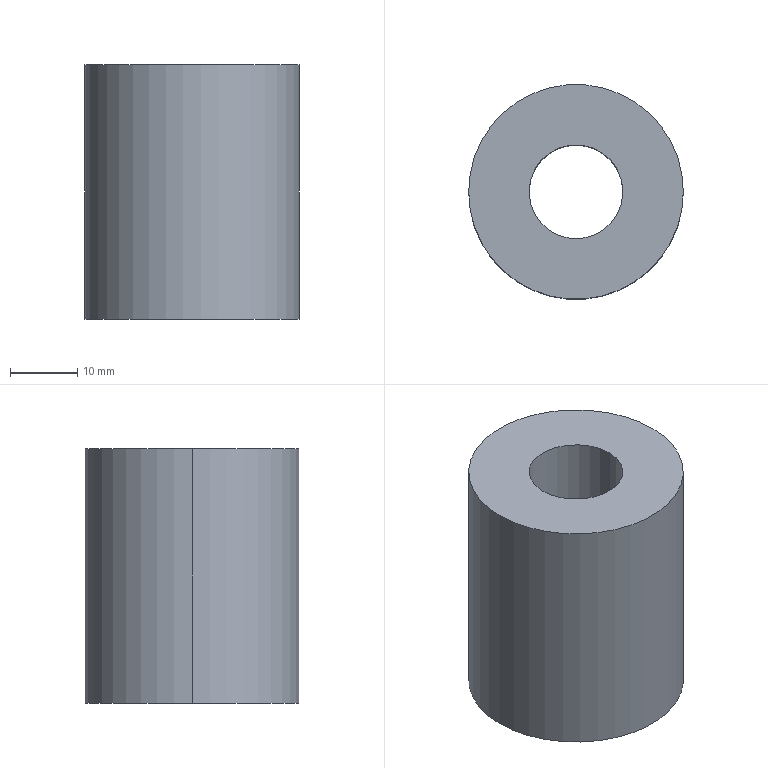Part | SolidWorks | features Extrusion 1, HoleWzd 1 | 1 solid | 6 faces | box 32 x 32 x 38 mm | volume 24712 mm3 | cylinder 4 | plane 2 | commonest cylinder face diameters 14 x2 32 x2
STEP:
#1=CARTESIAN_POINT('',(-7.,0.,0.));
#2=VERTEX_POINT('',#1);
#3=CARTESIAN_POINT('',(7.,0.,0.));
#4=VERTEX_POINT('',#3);
#5=CARTESIAN_POINT('',(0.,0.,0.));
#6=DIRECTION('',(0.,0.,1.));
#7=DIRECTION('',(1.,0.,0.));
#8=AXIS2_PLACEMENT_3D('',#5,#6,#7);
#9=CIRCLE('',#8,7.);
#10=EDGE_CURVE('',#2,#4,#9,.T.);
#11=ORIENTED_EDGE('',*,*,#10,.F.);
#12=CARTESIAN_POINT('',(-7.,0.,38.));
#13=VERTEX_POINT('',#12);
#14=CARTESIAN_POINT('',(-7.,0.,38.));
#15=DIRECTION('',(0.,0.,1.));
#16=VECTOR('',#15,1000.);
#17=LINE('',#14,#16);
#18=EDGE_CURVE('',#2,#13,#17,.T.);
#19=ORIENTED_EDGE('',*,*,#18,.T.);
#20=CARTESIAN_POINT('',(7.,0.,38.));
#21=VERTEX_POINT('',#20);
#22=CARTESIAN_POINT('',(0.,0.,38.));
#23=DIRECTION('',(0.,0.,1.));
#24=DIRECTION('',(1.,0.,0.));
#25=AXIS2_PLACEMENT_3D('',#22,#23,#24);
#26=CIRCLE('',#25,7.);
#27=EDGE_CURVE('',#13,#21,#26,.T.);
#28=ORIENTED_EDGE('',*,*,#27,.T.);
#29=CARTESIAN_POINT('',(7.,0.,38.));
#30=DIRECTION('',(0.,0.,1.));
#31=VECTOR('',#30,1000.);
#32=LINE('',#29,#31);
#33=EDGE_CURVE('',#4,#21,#32,.T.);
#34=ORIENTED_EDGE('',*,*,#33,.F.);
#35=EDGE_LOOP('',(#11,#19,#28,#34));
#36=FACE_OUTER_BOUND('',#35,.T.);
#37=CARTESIAN_POINT('',(0.,0.,38.));
#38=DIRECTION('',(0.,0.,1.));
#39=DIRECTION('',(1.,0.,0.));
#40=AXIS2_PLACEMENT_3D('',#37,#38,#39);
#41=CYLINDRICAL_SURFACE('',#40,7.);
#42=ADVANCED_FACE('',(#36),#41,.F.);
#43=CARTESIAN_POINT('',(16.,0.,38.));
#44=VERTEX_POINT('',#43);
#45=CARTESIAN_POINT('',(-16.,0.,38.));
#46=VERTEX_POINT('',#45);
#47=CARTESIAN_POINT('',(0.,0.,38.));
#48=DIRECTION('',(0.,0.,1.));
#49=DIRECTION('',(1.,0.,0.));
#50=AXIS2_PLACEMENT_3D('',#47,#48,#49);
#51=CIRCLE('',#50,16.);
#52=EDGE_CURVE('',#44,#46,#51,.T.);
#53=ORIENTED_EDGE('',*,*,#52,.F.);
#54=CARTESIAN_POINT('',(16.,0.,0.));
#55=VERTEX_POINT('',#54);
#56=CARTESIAN_POINT('',(16.,0.,38.));
#57=DIRECTION('',(0.,0.,-1.));
#58=VECTOR('',#57,1000.);
#59=LINE('',#56,#58);
#60=EDGE_CURVE('',#44,#55,#59,.T.);
#61=ORIENTED_EDGE('',*,*,#60,.T.);
#62=CARTESIAN_POINT('',(-16.,0.,0.));
#63=VERTEX_POINT('',#62);
#64=CARTESIAN_POINT('',(0.,0.,0.));
#65=DIRECTION('',(0.,0.,1.));
#66=DIRECTION('',(1.,0.,0.));
#67=AXIS2_PLACEMENT_3D('',#64,#65,#66);
#68=CIRCLE('',#67,16.);
#69=EDGE_CURVE('',#55,#63,#68,.T.);
#70=ORIENTED_EDGE('',*,*,#69,.T.);
#71=CARTESIAN_POINT('',(-16.,0.,38.));
#72=DIRECTION('',(0.,0.,-1.));
#73=VECTOR('',#72,1000.);
#74=LINE('',#71,#73);
#75=EDGE_CURVE('',#46,#63,#74,.T.);
#76=ORIENTED_EDGE('',*,*,#75,.F.);
#77=EDGE_LOOP('',(#53,#61,#70,#76));
#78=FACE_OUTER_BOUND('',#77,.T.);
#79=CARTESIAN_POINT('',(0.,0.,38.));
#80=DIRECTION('',(0.,0.,-1.));
#81=DIRECTION('',(-1.,0.,0.));
#82=AXIS2_PLACEMENT_3D('',#79,#80,#81);
#83=CYLINDRICAL_SURFACE('',#82,16.);
#84=ADVANCED_FACE('',(#78),#83,.T.);
#85=ORIENTED_EDGE('',*,*,#60,.F.);
#86=CARTESIAN_POINT('',(0.,0.,38.));
#87=DIRECTION('',(0.,0.,1.));
#88=DIRECTION('',(1.,0.,0.));
#89=AXIS2_PLACEMENT_3D('',#86,#87,#88);
#90=CIRCLE('',#89,16.);
#91=EDGE_CURVE('',#46,#44,#90,.T.);
#92=ORIENTED_EDGE('',*,*,#91,.F.);
#93=ORIENTED_EDGE('',*,*,#75,.T.);
#94=CARTESIAN_POINT('',(0.,0.,0.));
#95=DIRECTION('',(0.,0.,1.));
#96=DIRECTION('',(1.,0.,0.));
#97=AXIS2_PLACEMENT_3D('',#94,#95,#96);
#98=CIRCLE('',#97,16.);
#99=EDGE_CURVE('',#63,#55,#98,.T.);
#100=ORIENTED_EDGE('',*,*,#99,.T.);
#101=EDGE_LOOP('',(#85,#92,#93,#100));
#102=FACE_OUTER_BOUND('',#101,.T.);
#103=CARTESIAN_POINT('',(0.,0.,38.));
#104=DIRECTION('',(0.,0.,-1.));
#105=DIRECTION('',(-1.,0.,0.));
#106=AXIS2_PLACEMENT_3D('',#103,#104,#105);
#107=CYLINDRICAL_SURFACE('',#106,16.);
#108=ADVANCED_FACE('',(#102),#107,.T.);
#109=CARTESIAN_POINT('',(0.,0.,38.));
#110=DIRECTION('',(0.,0.,1.));
#111=DIRECTION('',(1.,0.,0.));
#112=AXIS2_PLACEMENT_3D('',#109,#110,#111);
#113=CIRCLE('',#112,7.);
#114=EDGE_CURVE('',#21,#13,#113,.T.);
#115=ORIENTED_EDGE('',*,*,#114,.F.);
#116=ORIENTED_EDGE('',*,*,#27,.F.);
#117=EDGE_LOOP('',(#115,#116));
#118=FACE_BOUND('',#117,.T.);
#119=ORIENTED_EDGE('',*,*,#91,.T.);
#120=ORIENTED_EDGE('',*,*,#52,.T.);
#121=EDGE_LOOP('',(#119,#120));
#122=FACE_OUTER_BOUND('',#121,.T.);
#123=CARTESIAN_POINT('',(0.,0.,38.));
#124=DIRECTION('',(0.,0.,1.));
#125=DIRECTION('',(1.,0.,0.));
#126=AXIS2_PLACEMENT_3D('',#123,#124,#125);
#127=PLANE('',#126);
#128=ADVANCED_FACE('',(#118,#122),#127,.T.);
#129=CARTESIAN_POINT('',(0.,0.,0.));
#130=DIRECTION('',(0.,0.,1.));
#131=DIRECTION('',(1.,0.,0.));
#132=AXIS2_PLACEMENT_3D('',#129,#130,#131);
#133=CIRCLE('',#132,7.);
#134=EDGE_CURVE('',#4,#2,#133,.T.);
#135=ORIENTED_EDGE('',*,*,#134,.T.);
#136=ORIENTED_EDGE('',*,*,#10,.T.);
#137=EDGE_LOOP('',(#135,#136));
#138=FACE_BOUND('',#137,.T.);
#139=ORIENTED_EDGE('',*,*,#99,.F.);
#140=ORIENTED_EDGE('',*,*,#69,.F.);
#141=EDGE_LOOP('',(#139,#140));
#142=FACE_OUTER_BOUND('',#141,.T.);
#143=CARTESIAN_POINT('',(0.,0.,0.));
#144=DIRECTION('',(0.,0.,1.));
#145=DIRECTION('',(1.,0.,0.));
#146=AXIS2_PLACEMENT_3D('',#143,#144,#145);
#147=PLANE('',#146);
#148=ADVANCED_FACE('',(#138,#142),#147,.F.);
#149=ORIENTED_EDGE('',*,*,#18,.F.);
#150=ORIENTED_EDGE('',*,*,#134,.F.);
#151=ORIENTED_EDGE('',*,*,#33,.T.);
#152=ORIENTED_EDGE('',*,*,#114,.T.);
#153=EDGE_LOOP('',(#149,#150,#151,#152));
#154=FACE_OUTER_BOUND('',#153,.T.);
#155=CARTESIAN_POINT('',(0.,0.,38.));
#156=DIRECTION('',(0.,0.,1.));
#157=DIRECTION('',(1.,0.,0.));
#158=AXIS2_PLACEMENT_3D('',#155,#156,#157);
#159=CYLINDRICAL_SURFACE('',#158,7.);
#160=ADVANCED_FACE('',(#154),#159,.F.);
#161=CLOSED_SHELL('',(#42,#84,#108,#128,#148,#160));
#162=MANIFOLD_SOLID_BREP('',#161);
#163=CARTESIAN_POINT('',(0.,0.,0.));
#164=DIRECTION('',(0.,0.,1.));
#165=DIRECTION('',(1.,0.,0.));
#166=AXIS2_PLACEMENT_3D('',#163,#164,#165);
#167=(LENGTH_UNIT()NAMED_UNIT(*)SI_UNIT(.MILLI.,.METRE.));
#168=UNCERTAINTY_MEASURE_WITH_UNIT(LENGTH_MEASURE(0.00001),#167,'','');
#169=(NAMED_UNIT(*)PLANE_ANGLE_UNIT()SI_UNIT($,.RADIAN.));
#170=(NAMED_UNIT(*)SI_UNIT($,.STERADIAN.)SOLID_ANGLE_UNIT());
#171=(GEOMETRIC_REPRESENTATION_CONTEXT(3)GLOBAL_UNCERTAINTY_ASSIGNED_CONTEXT((#168))GLOBAL_UNIT_ASSIGNED_CONTEXT((#167,#169,#170))REPRESENTATION_CONTEXT('',''));
#172=ADVANCED_BREP_SHAPE_REPRESENTATION('',(#162,#166),#171);